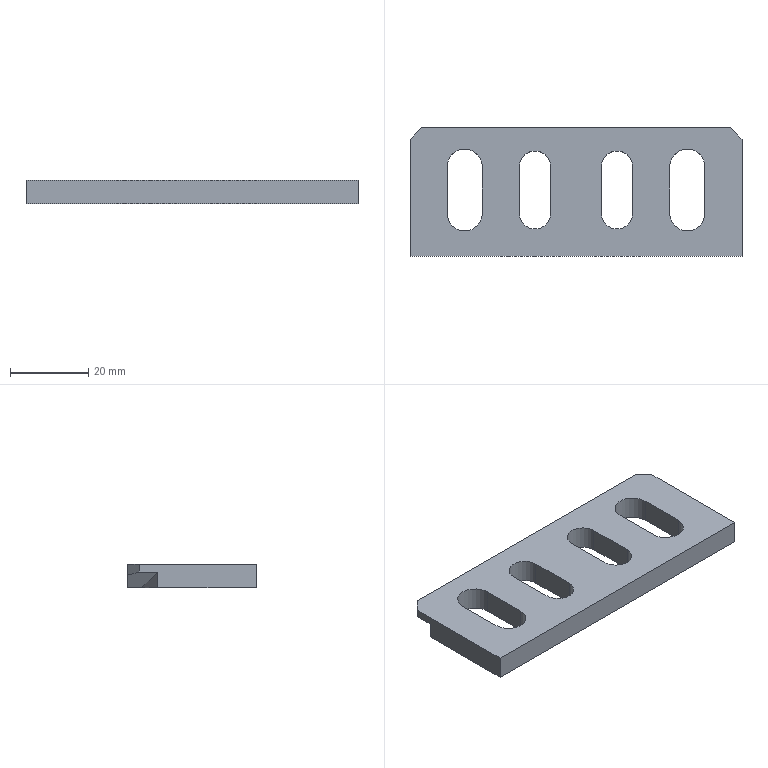Part | STEP file | gslz 2016.10.28-13_id1598_x_t | 1 solid | 29 faces | box 85 x 33 x 6 mm | volume 12707 mm3 | plane 21 | cylinder 8 | commonest cylinder face diameters 8 x4 9 x4